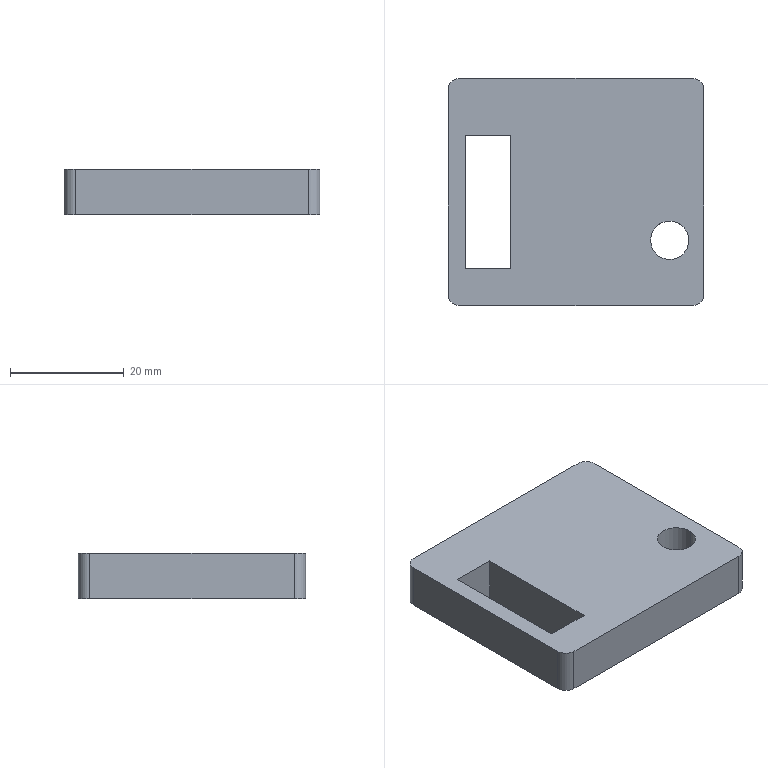Part | SolidWorks | features Fillet 1, FlatPattern 1, SMBaseFlange 1, SheetMetal 1 | 1 solid | 16 faces | box 45 x 40 x 8 mm | volume 12582 mm3 | plane 10 | cylinder 6 | commonest cylinder face diameters 4 x4 6.75 x2
STEP:
#1=CARTESIAN_POINT('',(-158.375,325.,8.));
#2=VERTEX_POINT('',#1);
#3=CARTESIAN_POINT('',(-151.625,325.,8.));
#4=VERTEX_POINT('',#3);
#5=CARTESIAN_POINT('',(-155.,325.,8.));
#6=DIRECTION('',(0.,0.,1.));
#7=DIRECTION('',(1.,0.,0.));
#8=AXIS2_PLACEMENT_3D('',#5,#6,#7);
#9=CIRCLE('',#8,3.375);
#10=EDGE_CURVE('',#2,#4,#9,.T.);
#11=ORIENTED_EDGE('',*,*,#10,.T.);
#12=CARTESIAN_POINT('',(-151.625,325.,0.));
#13=VERTEX_POINT('',#12);
#14=CARTESIAN_POINT('',(-151.625,325.,8.));
#15=DIRECTION('',(0.,0.,-1.));
#16=VECTOR('',#15,1000.);
#17=LINE('',#14,#16);
#18=EDGE_CURVE('',#4,#13,#17,.T.);
#19=ORIENTED_EDGE('',*,*,#18,.T.);
#20=CARTESIAN_POINT('',(-158.375,325.,0.));
#21=VERTEX_POINT('',#20);
#22=CARTESIAN_POINT('',(-155.,325.,0.));
#23=DIRECTION('',(0.,0.,1.));
#24=DIRECTION('',(1.,0.,0.));
#25=AXIS2_PLACEMENT_3D('',#22,#23,#24);
#26=CIRCLE('',#25,3.375);
#27=EDGE_CURVE('',#21,#13,#26,.T.);
#28=ORIENTED_EDGE('',*,*,#27,.F.);
#29=CARTESIAN_POINT('',(-158.375,325.,8.));
#30=DIRECTION('',(0.,0.,-1.));
#31=VECTOR('',#30,1000.);
#32=LINE('',#29,#31);
#33=EDGE_CURVE('',#2,#21,#32,.T.);
#34=ORIENTED_EDGE('',*,*,#33,.F.);
#35=EDGE_LOOP('',(#11,#19,#28,#34));
#36=FACE_OUTER_BOUND('',#35,.T.);
#37=CARTESIAN_POINT('',(-155.,325.,8.));
#38=DIRECTION('',(0.,0.,-1.));
#39=DIRECTION('',(-1.,0.,0.));
#40=AXIS2_PLACEMENT_3D('',#37,#38,#39);
#41=CYLINDRICAL_SURFACE('',#40,3.375);
#42=ADVANCED_FACE('',(#36),#41,.F.);
#43=CARTESIAN_POINT('',(-149.,315.5,8.));
#44=VERTEX_POINT('',#43);
#45=CARTESIAN_POINT('',(-149.,351.5,8.));
#46=VERTEX_POINT('',#45);
#47=CARTESIAN_POINT('',(-149.,313.5,8.));
#48=DIRECTION('',(0.,1.,0.));
#49=VECTOR('',#48,1000.);
#50=LINE('',#47,#49);
#51=EDGE_CURVE('',#44,#46,#50,.T.);
#52=ORIENTED_EDGE('',*,*,#51,.T.);
#53=CARTESIAN_POINT('',(-151.,353.5,8.));
#54=VERTEX_POINT('',#53);
#55=CARTESIAN_POINT('',(-151.,351.5,8.));
#56=DIRECTION('',(0.,0.,1.));
#57=DIRECTION('',(1.,0.,0.));
#58=AXIS2_PLACEMENT_3D('',#55,#56,#57);
#59=CIRCLE('',#58,2.);
#60=EDGE_CURVE('',#46,#54,#59,.T.);
#61=ORIENTED_EDGE('',*,*,#60,.T.);
#62=CARTESIAN_POINT('',(-192.,353.5,8.));
#63=VERTEX_POINT('',#62);
#64=CARTESIAN_POINT('',(-149.,353.5,8.));
#65=DIRECTION('',(-1.,0.,0.));
#66=VECTOR('',#65,1000.);
#67=LINE('',#64,#66);
#68=EDGE_CURVE('',#54,#63,#67,.T.);
#69=ORIENTED_EDGE('',*,*,#68,.T.);
#70=CARTESIAN_POINT('',(-194.,351.5,8.));
#71=VERTEX_POINT('',#70);
#72=CARTESIAN_POINT('',(-192.,351.5,8.));
#73=DIRECTION('',(0.,0.,1.));
#74=DIRECTION('',(1.,0.,0.));
#75=AXIS2_PLACEMENT_3D('',#72,#73,#74);
#76=CIRCLE('',#75,2.);
#77=EDGE_CURVE('',#63,#71,#76,.T.);
#78=ORIENTED_EDGE('',*,*,#77,.T.);
#79=CARTESIAN_POINT('',(-194.,315.5,8.));
#80=VERTEX_POINT('',#79);
#81=CARTESIAN_POINT('',(-194.,353.5,8.));
#82=DIRECTION('',(0.,-1.,0.));
#83=VECTOR('',#82,1000.);
#84=LINE('',#81,#83);
#85=EDGE_CURVE('',#71,#80,#84,.T.);
#86=ORIENTED_EDGE('',*,*,#85,.T.);
#87=CARTESIAN_POINT('',(-192.,313.5,8.));
#88=VERTEX_POINT('',#87);
#89=CARTESIAN_POINT('',(-192.,315.5,8.));
#90=DIRECTION('',(0.,0.,1.));
#91=DIRECTION('',(1.,0.,0.));
#92=AXIS2_PLACEMENT_3D('',#89,#90,#91);
#93=CIRCLE('',#92,2.);
#94=EDGE_CURVE('',#80,#88,#93,.T.);
#95=ORIENTED_EDGE('',*,*,#94,.T.);
#96=CARTESIAN_POINT('',(-151.,313.5,8.));
#97=VERTEX_POINT('',#96);
#98=CARTESIAN_POINT('',(-194.,313.5,8.));
#99=DIRECTION('',(1.,0.,0.));
#100=VECTOR('',#99,1000.);
#101=LINE('',#98,#100);
#102=EDGE_CURVE('',#88,#97,#101,.T.);
#103=ORIENTED_EDGE('',*,*,#102,.T.);
#104=CARTESIAN_POINT('',(-151.,315.5,8.));
#105=DIRECTION('',(0.,0.,1.));
#106=DIRECTION('',(1.,0.,0.));
#107=AXIS2_PLACEMENT_3D('',#104,#105,#106);
#108=CIRCLE('',#107,2.);
#109=EDGE_CURVE('',#97,#44,#108,.T.);
#110=ORIENTED_EDGE('',*,*,#109,.T.);
#111=EDGE_LOOP('',(#52,#61,#69,#78,#86,#95,#103,#110));
#112=FACE_OUTER_BOUND('',#111,.T.);
#113=ORIENTED_EDGE('',*,*,#10,.F.);
#114=CARTESIAN_POINT('',(-155.,325.,8.));
#115=DIRECTION('',(0.,0.,1.));
#116=DIRECTION('',(1.,0.,0.));
#117=AXIS2_PLACEMENT_3D('',#114,#115,#116);
#118=CIRCLE('',#117,3.375);
#119=EDGE_CURVE('',#4,#2,#118,.T.);
#120=ORIENTED_EDGE('',*,*,#119,.F.);
#121=EDGE_LOOP('',(#113,#120));
#122=FACE_BOUND('',#121,.T.);
#123=CARTESIAN_POINT('',(-191.,320.,8.));
#124=VERTEX_POINT('',#123);
#125=CARTESIAN_POINT('',(-183.,320.,8.));
#126=VERTEX_POINT('',#125);
#127=CARTESIAN_POINT('',(-183.,320.,8.));
#128=DIRECTION('',(1.,0.,0.));
#129=VECTOR('',#128,1000.);
#130=LINE('',#127,#129);
#131=EDGE_CURVE('',#124,#126,#130,.T.);
#132=ORIENTED_EDGE('',*,*,#131,.F.);
#133=CARTESIAN_POINT('',(-191.,343.5,8.));
#134=VERTEX_POINT('',#133);
#135=CARTESIAN_POINT('',(-191.,320.,8.));
#136=DIRECTION('',(0.,-1.,0.));
#137=VECTOR('',#136,1000.);
#138=LINE('',#135,#137);
#139=EDGE_CURVE('',#134,#124,#138,.T.);
#140=ORIENTED_EDGE('',*,*,#139,.F.);
#141=CARTESIAN_POINT('',(-183.,343.5,8.));
#142=VERTEX_POINT('',#141);
#143=CARTESIAN_POINT('',(-191.,343.5,8.));
#144=DIRECTION('',(-1.,0.,0.));
#145=VECTOR('',#144,1000.);
#146=LINE('',#143,#145);
#147=EDGE_CURVE('',#142,#134,#146,.T.);
#148=ORIENTED_EDGE('',*,*,#147,.F.);
#149=CARTESIAN_POINT('',(-183.,343.5,8.));
#150=DIRECTION('',(0.,1.,0.));
#151=VECTOR('',#150,1000.);
#152=LINE('',#149,#151);
#153=EDGE_CURVE('',#126,#142,#152,.T.);
#154=ORIENTED_EDGE('',*,*,#153,.F.);
#155=EDGE_LOOP('',(#132,#140,#148,#154));
#156=FACE_BOUND('',#155,.T.);
#157=CARTESIAN_POINT('',(0.,0.,8.));
#158=DIRECTION('',(0.,0.,1.));
#159=DIRECTION('',(1.,0.,0.));
#160=AXIS2_PLACEMENT_3D('',#157,#158,#159);
#161=PLANE('',#160);
#162=ADVANCED_FACE('',(#112,#122,#156),#161,.T.);
#163=ORIENTED_EDGE('',*,*,#27,.T.);
#164=CARTESIAN_POINT('',(-155.,325.,0.));
#165=DIRECTION('',(0.,0.,1.));
#166=DIRECTION('',(1.,0.,0.));
#167=AXIS2_PLACEMENT_3D('',#164,#165,#166);
#168=CIRCLE('',#167,3.375);
#169=EDGE_CURVE('',#13,#21,#168,.T.);
#170=ORIENTED_EDGE('',*,*,#169,.T.);
#171=EDGE_LOOP('',(#163,#170));
#172=FACE_BOUND('',#171,.T.);
#173=CARTESIAN_POINT('',(-151.,353.5,0.));
#174=VERTEX_POINT('',#173);
#175=CARTESIAN_POINT('',(-192.,353.5,0.));
#176=VERTEX_POINT('',#175);
#177=CARTESIAN_POINT('',(-149.,353.5,0.));
#178=DIRECTION('',(-1.,0.,0.));
#179=VECTOR('',#178,1000.);
#180=LINE('',#177,#179);
#181=EDGE_CURVE('',#174,#176,#180,.T.);
#182=ORIENTED_EDGE('',*,*,#181,.F.);
#183=CARTESIAN_POINT('',(-149.,351.5,0.));
#184=VERTEX_POINT('',#183);
#185=CARTESIAN_POINT('',(-151.,351.5,0.));
#186=DIRECTION('',(0.,0.,-1.));
#187=DIRECTION('',(1.,0.,0.));
#188=AXIS2_PLACEMENT_3D('',#185,#186,#187);
#189=CIRCLE('',#188,2.);
#190=EDGE_CURVE('',#174,#184,#189,.T.);
#191=ORIENTED_EDGE('',*,*,#190,.T.);
#192=CARTESIAN_POINT('',(-149.,315.5,0.));
#193=VERTEX_POINT('',#192);
#194=CARTESIAN_POINT('',(-149.,313.5,0.));
#195=DIRECTION('',(0.,1.,0.));
#196=VECTOR('',#195,1000.);
#197=LINE('',#194,#196);
#198=EDGE_CURVE('',#193,#184,#197,.T.);
#199=ORIENTED_EDGE('',*,*,#198,.F.);
#200=CARTESIAN_POINT('',(-151.,313.5,0.));
#201=VERTEX_POINT('',#200);
#202=CARTESIAN_POINT('',(-151.,315.5,0.));
#203=DIRECTION('',(0.,0.,-1.));
#204=DIRECTION('',(1.,0.,0.));
#205=AXIS2_PLACEMENT_3D('',#202,#203,#204);
#206=CIRCLE('',#205,2.);
#207=EDGE_CURVE('',#193,#201,#206,.T.);
#208=ORIENTED_EDGE('',*,*,#207,.T.);
#209=CARTESIAN_POINT('',(-192.,313.5,0.));
#210=VERTEX_POINT('',#209);
#211=CARTESIAN_POINT('',(-194.,313.5,0.));
#212=DIRECTION('',(1.,0.,0.));
#213=VECTOR('',#212,1000.);
#214=LINE('',#211,#213);
#215=EDGE_CURVE('',#210,#201,#214,.T.);
#216=ORIENTED_EDGE('',*,*,#215,.F.);
#217=CARTESIAN_POINT('',(-194.,315.5,0.));
#218=VERTEX_POINT('',#217);
#219=CARTESIAN_POINT('',(-192.,315.5,0.));
#220=DIRECTION('',(0.,0.,-1.));
#221=DIRECTION('',(1.,0.,0.));
#222=AXIS2_PLACEMENT_3D('',#219,#220,#221);
#223=CIRCLE('',#222,2.);
#224=EDGE_CURVE('',#210,#218,#223,.T.);
#225=ORIENTED_EDGE('',*,*,#224,.T.);
#226=CARTESIAN_POINT('',(-194.,351.5,0.));
#227=VERTEX_POINT('',#226);
#228=CARTESIAN_POINT('',(-194.,353.5,0.));
#229=DIRECTION('',(0.,-1.,0.));
#230=VECTOR('',#229,1000.);
#231=LINE('',#228,#230);
#232=EDGE_CURVE('',#227,#218,#231,.T.);
#233=ORIENTED_EDGE('',*,*,#232,.F.);
#234=CARTESIAN_POINT('',(-192.,351.5,0.));
#235=DIRECTION('',(0.,0.,-1.));
#236=DIRECTION('',(1.,0.,0.));
#237=AXIS2_PLACEMENT_3D('',#234,#235,#236);
#238=CIRCLE('',#237,2.);
#239=EDGE_CURVE('',#227,#176,#238,.T.);
#240=ORIENTED_EDGE('',*,*,#239,.T.);
#241=EDGE_LOOP('',(#182,#191,#199,#208,#216,#225,#233,#240));
#242=FACE_OUTER_BOUND('',#241,.T.);
#243=CARTESIAN_POINT('',(-191.,343.5,0.));
#244=VERTEX_POINT('',#243);
#245=CARTESIAN_POINT('',(-191.,320.,0.));
#246=VERTEX_POINT('',#245);
#247=CARTESIAN_POINT('',(-191.,320.,0.));
#248=DIRECTION('',(0.,-1.,0.));
#249=VECTOR('',#248,1000.);
#250=LINE('',#247,#249);
#251=EDGE_CURVE('',#244,#246,#250,.T.);
#252=ORIENTED_EDGE('',*,*,#251,.T.);
#253=CARTESIAN_POINT('',(-183.,320.,0.));
#254=VERTEX_POINT('',#253);
#255=CARTESIAN_POINT('',(-183.,320.,0.));
#256=DIRECTION('',(1.,0.,0.));
#257=VECTOR('',#256,1000.);
#258=LINE('',#255,#257);
#259=EDGE_CURVE('',#246,#254,#258,.T.);
#260=ORIENTED_EDGE('',*,*,#259,.T.);
#261=CARTESIAN_POINT('',(-183.,343.5,0.));
#262=VERTEX_POINT('',#261);
#263=CARTESIAN_POINT('',(-183.,343.5,0.));
#264=DIRECTION('',(0.,1.,0.));
#265=VECTOR('',#264,1000.);
#266=LINE('',#263,#265);
#267=EDGE_CURVE('',#254,#262,#266,.T.);
#268=ORIENTED_EDGE('',*,*,#267,.T.);
#269=CARTESIAN_POINT('',(-191.,343.5,0.));
#270=DIRECTION('',(-1.,0.,0.));
#271=VECTOR('',#270,1000.);
#272=LINE('',#269,#271);
#273=EDGE_CURVE('',#262,#244,#272,.T.);
#274=ORIENTED_EDGE('',*,*,#273,.T.);
#275=EDGE_LOOP('',(#252,#260,#268,#274));
#276=FACE_BOUND('',#275,.T.);
#277=CARTESIAN_POINT('',(0.,0.,0.));
#278=DIRECTION('',(0.,0.,1.));
#279=DIRECTION('',(1.,0.,0.));
#280=AXIS2_PLACEMENT_3D('',#277,#278,#279);
#281=PLANE('',#280);
#282=ADVANCED_FACE('',(#172,#242,#276),#281,.F.);
#283=ORIENTED_EDGE('',*,*,#232,.T.);
#284=CARTESIAN_POINT('',(-194.,315.5,8.));
#285=DIRECTION('',(0.,0.,1.));
#286=VECTOR('',#285,1000.);
#287=LINE('',#284,#286);
#288=EDGE_CURVE('',#218,#80,#287,.T.);
#289=ORIENTED_EDGE('',*,*,#288,.T.);
#290=ORIENTED_EDGE('',*,*,#85,.F.);
#291=CARTESIAN_POINT('',(-194.,351.5,8.));
#292=DIRECTION('',(0.,0.,-1.));
#293=VECTOR('',#292,1000.);
#294=LINE('',#291,#293);
#295=EDGE_CURVE('',#71,#227,#294,.T.);
#296=ORIENTED_EDGE('',*,*,#295,.T.);
#297=EDGE_LOOP('',(#283,#289,#290,#296));
#298=FACE_OUTER_BOUND('',#297,.T.);
#299=CARTESIAN_POINT('',(-194.,353.5,8.));
#300=DIRECTION('',(1.,0.,0.));
#301=DIRECTION('',(0.,1.,0.));
#302=AXIS2_PLACEMENT_3D('',#299,#300,#301);
#303=PLANE('',#302);
#304=ADVANCED_FACE('',(#298),#303,.F.);
#305=ORIENTED_EDGE('',*,*,#215,.T.);
#306=CARTESIAN_POINT('',(-151.,313.5,8.));
#307=DIRECTION('',(0.,0.,1.));
#308=VECTOR('',#307,1000.);
#309=LINE('',#306,#308);
#310=EDGE_CURVE('',#201,#97,#309,.T.);
#311=ORIENTED_EDGE('',*,*,#310,.T.);
#312=ORIENTED_EDGE('',*,*,#102,.F.);
#313=CARTESIAN_POINT('',(-192.,313.5,8.));
#314=DIRECTION('',(0.,0.,-1.));
#315=VECTOR('',#314,1000.);
#316=LINE('',#313,#315);
#317=EDGE_CURVE('',#88,#210,#316,.T.);
#318=ORIENTED_EDGE('',*,*,#317,.T.);
#319=EDGE_LOOP('',(#305,#311,#312,#318));
#320=FACE_OUTER_BOUND('',#319,.T.);
#321=CARTESIAN_POINT('',(-194.,313.5,8.));
#322=DIRECTION('',(0.,1.,0.));
#323=DIRECTION('',(0.,0.,1.));
#324=AXIS2_PLACEMENT_3D('',#321,#322,#323);
#325=PLANE('',#324);
#326=ADVANCED_FACE('',(#320),#325,.F.);
#327=ORIENTED_EDGE('',*,*,#198,.T.);
#328=CARTESIAN_POINT('',(-149.,351.5,8.));
#329=DIRECTION('',(0.,0.,1.));
#330=VECTOR('',#329,1000.);
#331=LINE('',#328,#330);
#332=EDGE_CURVE('',#184,#46,#331,.T.);
#333=ORIENTED_EDGE('',*,*,#332,.T.);
#334=ORIENTED_EDGE('',*,*,#51,.F.);
#335=CARTESIAN_POINT('',(-149.,315.5,8.));
#336=DIRECTION('',(0.,0.,-1.));
#337=VECTOR('',#336,1000.);
#338=LINE('',#335,#337);
#339=EDGE_CURVE('',#44,#193,#338,.T.);
#340=ORIENTED_EDGE('',*,*,#339,.T.);
#341=EDGE_LOOP('',(#327,#333,#334,#340));
#342=FACE_OUTER_BOUND('',#341,.T.);
#343=CARTESIAN_POINT('',(-149.,313.5,8.));
#344=DIRECTION('',(-1.,0.,0.));
#345=DIRECTION('',(0.,0.,1.));
#346=AXIS2_PLACEMENT_3D('',#343,#344,#345);
#347=PLANE('',#346);
#348=ADVANCED_FACE('',(#342),#347,.F.);
#349=ORIENTED_EDGE('',*,*,#68,.F.);
#350=CARTESIAN_POINT('',(-151.,353.5,8.));
#351=DIRECTION('',(0.,0.,-1.));
#352=VECTOR('',#351,1000.);
#353=LINE('',#350,#352);
#354=EDGE_CURVE('',#54,#174,#353,.T.);
#355=ORIENTED_EDGE('',*,*,#354,.T.);
#356=ORIENTED_EDGE('',*,*,#181,.T.);
#357=CARTESIAN_POINT('',(-192.,353.5,8.));
#358=DIRECTION('',(0.,0.,1.));
#359=VECTOR('',#358,1000.);
#360=LINE('',#357,#359);
#361=EDGE_CURVE('',#176,#63,#360,.T.);
#362=ORIENTED_EDGE('',*,*,#361,.T.);
#363=EDGE_LOOP('',(#349,#355,#356,#362));
#364=FACE_OUTER_BOUND('',#363,.T.);
#365=CARTESIAN_POINT('',(-149.,353.5,8.));
#366=DIRECTION('',(0.,-1.,0.));
#367=DIRECTION('',(0.,0.,-1.));
#368=AXIS2_PLACEMENT_3D('',#365,#366,#367);
#369=PLANE('',#368);
#370=ADVANCED_FACE('',(#364),#369,.F.);
#371=ORIENTED_EDGE('',*,*,#18,.F.);
#372=ORIENTED_EDGE('',*,*,#119,.T.);
#373=ORIENTED_EDGE('',*,*,#33,.T.);
#374=ORIENTED_EDGE('',*,*,#169,.F.);
#375=EDGE_LOOP('',(#371,#372,#373,#374));
#376=FACE_OUTER_BOUND('',#375,.T.);
#377=CARTESIAN_POINT('',(-155.,325.,8.));
#378=DIRECTION('',(0.,0.,-1.));
#379=DIRECTION('',(-1.,0.,0.));
#380=AXIS2_PLACEMENT_3D('',#377,#378,#379);
#381=CYLINDRICAL_SURFACE('',#380,3.375);
#382=ADVANCED_FACE('',(#376),#381,.F.);
#383=ORIENTED_EDGE('',*,*,#251,.F.);
#384=CARTESIAN_POINT('',(-191.,343.5,8.));
#385=DIRECTION('',(0.,0.,-1.));
#386=VECTOR('',#385,1000.);
#387=LINE('',#384,#386);
#388=EDGE_CURVE('',#134,#244,#387,.T.);
#389=ORIENTED_EDGE('',*,*,#388,.F.);
#390=ORIENTED_EDGE('',*,*,#139,.T.);
#391=CARTESIAN_POINT('',(-191.,320.,8.));
#392=DIRECTION('',(0.,0.,-1.));
#393=VECTOR('',#392,1000.);
#394=LINE('',#391,#393);
#395=EDGE_CURVE('',#124,#246,#394,.T.);
#396=ORIENTED_EDGE('',*,*,#395,.T.);
#397=EDGE_LOOP('',(#383,#389,#390,#396));
#398=FACE_OUTER_BOUND('',#397,.T.);
#399=CARTESIAN_POINT('',(-191.,320.,8.));
#400=DIRECTION('',(1.,0.,0.));
#401=DIRECTION('',(0.,0.,-1.));
#402=AXIS2_PLACEMENT_3D('',#399,#400,#401);
#403=PLANE('',#402);
#404=ADVANCED_FACE('',(#398),#403,.T.);
#405=ORIENTED_EDGE('',*,*,#259,.F.);
#406=ORIENTED_EDGE('',*,*,#395,.F.);
#407=ORIENTED_EDGE('',*,*,#131,.T.);
#408=CARTESIAN_POINT('',(-183.,320.,8.));
#409=DIRECTION('',(0.,0.,-1.));
#410=VECTOR('',#409,1000.);
#411=LINE('',#408,#410);
#412=EDGE_CURVE('',#126,#254,#411,.T.);
#413=ORIENTED_EDGE('',*,*,#412,.T.);
#414=EDGE_LOOP('',(#405,#406,#407,#413));
#415=FACE_OUTER_BOUND('',#414,.T.);
#416=CARTESIAN_POINT('',(-183.,320.,8.));
#417=DIRECTION('',(0.,1.,0.));
#418=DIRECTION('',(0.,0.,1.));
#419=AXIS2_PLACEMENT_3D('',#416,#417,#418);
#420=PLANE('',#419);
#421=ADVANCED_FACE('',(#415),#420,.T.);
#422=ORIENTED_EDGE('',*,*,#267,.F.);
#423=ORIENTED_EDGE('',*,*,#412,.F.);
#424=ORIENTED_EDGE('',*,*,#153,.T.);
#425=CARTESIAN_POINT('',(-183.,343.5,8.));
#426=DIRECTION('',(0.,0.,-1.));
#427=VECTOR('',#426,1000.);
#428=LINE('',#425,#427);
#429=EDGE_CURVE('',#142,#262,#428,.T.);
#430=ORIENTED_EDGE('',*,*,#429,.T.);
#431=EDGE_LOOP('',(#422,#423,#424,#430));
#432=FACE_OUTER_BOUND('',#431,.T.);
#433=CARTESIAN_POINT('',(-183.,343.5,8.));
#434=DIRECTION('',(-1.,0.,0.));
#435=DIRECTION('',(0.,0.,1.));
#436=AXIS2_PLACEMENT_3D('',#433,#434,#435);
#437=PLANE('',#436);
#438=ADVANCED_FACE('',(#432),#437,.T.);
#439=ORIENTED_EDGE('',*,*,#273,.F.);
#440=ORIENTED_EDGE('',*,*,#429,.F.);
#441=ORIENTED_EDGE('',*,*,#147,.T.);
#442=ORIENTED_EDGE('',*,*,#388,.T.);
#443=EDGE_LOOP('',(#439,#440,#441,#442));
#444=FACE_OUTER_BOUND('',#443,.T.);
#445=CARTESIAN_POINT('',(-191.,343.5,8.));
#446=DIRECTION('',(0.,-1.,0.));
#447=DIRECTION('',(0.,0.,-1.));
#448=AXIS2_PLACEMENT_3D('',#445,#446,#447);
#449=PLANE('',#448);
#450=ADVANCED_FACE('',(#444),#449,.T.);
#451=ORIENTED_EDGE('',*,*,#60,.F.);
#452=ORIENTED_EDGE('',*,*,#332,.F.);
#453=ORIENTED_EDGE('',*,*,#190,.F.);
#454=ORIENTED_EDGE('',*,*,#354,.F.);
#455=EDGE_LOOP('',(#451,#452,#453,#454));
#456=FACE_OUTER_BOUND('',#455,.T.);
#457=CARTESIAN_POINT('',(-151.,351.5,8.));
#458=DIRECTION('',(0.,0.,-1.));
#459=DIRECTION('',(-1.,0.,0.));
#460=AXIS2_PLACEMENT_3D('',#457,#458,#459);
#461=CYLINDRICAL_SURFACE('',#460,2.);
#462=ADVANCED_FACE('',(#456),#461,.T.);
#463=ORIENTED_EDGE('',*,*,#109,.F.);
#464=ORIENTED_EDGE('',*,*,#310,.F.);
#465=ORIENTED_EDGE('',*,*,#207,.F.);
#466=ORIENTED_EDGE('',*,*,#339,.F.);
#467=EDGE_LOOP('',(#463,#464,#465,#466));
#468=FACE_OUTER_BOUND('',#467,.T.);
#469=CARTESIAN_POINT('',(-151.,315.5,8.));
#470=DIRECTION('',(0.,0.,-1.));
#471=DIRECTION('',(-1.,0.,0.));
#472=AXIS2_PLACEMENT_3D('',#469,#470,#471);
#473=CYLINDRICAL_SURFACE('',#472,2.);
#474=ADVANCED_FACE('',(#468),#473,.T.);
#475=ORIENTED_EDGE('',*,*,#94,.F.);
#476=ORIENTED_EDGE('',*,*,#288,.F.);
#477=ORIENTED_EDGE('',*,*,#224,.F.);
#478=ORIENTED_EDGE('',*,*,#317,.F.);
#479=EDGE_LOOP('',(#475,#476,#477,#478));
#480=FACE_OUTER_BOUND('',#479,.T.);
#481=CARTESIAN_POINT('',(-192.,315.5,8.));
#482=DIRECTION('',(0.,0.,-1.));
#483=DIRECTION('',(-1.,0.,0.));
#484=AXIS2_PLACEMENT_3D('',#481,#482,#483);
#485=CYLINDRICAL_SURFACE('',#484,2.);
#486=ADVANCED_FACE('',(#480),#485,.T.);
#487=ORIENTED_EDGE('',*,*,#77,.F.);
#488=ORIENTED_EDGE('',*,*,#361,.F.);
#489=ORIENTED_EDGE('',*,*,#239,.F.);
#490=ORIENTED_EDGE('',*,*,#295,.F.);
#491=EDGE_LOOP('',(#487,#488,#489,#490));
#492=FACE_OUTER_BOUND('',#491,.T.);
#493=CARTESIAN_POINT('',(-192.,351.5,8.));
#494=DIRECTION('',(0.,0.,-1.));
#495=DIRECTION('',(-1.,0.,0.));
#496=AXIS2_PLACEMENT_3D('',#493,#494,#495);
#497=CYLINDRICAL_SURFACE('',#496,2.);
#498=ADVANCED_FACE('',(#492),#497,.T.);
#499=CLOSED_SHELL('',(#42,#162,#282,#304,#326,#348,#370,#382,#404,#421,#438,#450,#462,#474,#486,#498));
#500=MANIFOLD_SOLID_BREP('',#499);
#501=CARTESIAN_POINT('',(0.,0.,0.));
#502=DIRECTION('',(0.,0.,1.));
#503=DIRECTION('',(1.,0.,0.));
#504=AXIS2_PLACEMENT_3D('',#501,#502,#503);
#505=(LENGTH_UNIT()NAMED_UNIT(*)SI_UNIT(.MILLI.,.METRE.));
#506=UNCERTAINTY_MEASURE_WITH_UNIT(LENGTH_MEASURE(0.00001),#505,'','');
#507=(NAMED_UNIT(*)PLANE_ANGLE_UNIT()SI_UNIT($,.RADIAN.));
#508=(NAMED_UNIT(*)SI_UNIT($,.STERADIAN.)SOLID_ANGLE_UNIT());
#509=(GEOMETRIC_REPRESENTATION_CONTEXT(3)GLOBAL_UNCERTAINTY_ASSIGNED_CONTEXT((#506))GLOBAL_UNIT_ASSIGNED_CONTEXT((#505,#507,#508))REPRESENTATION_CONTEXT('',''));
#510=ADVANCED_BREP_SHAPE_REPRESENTATION('',(#500,#504),#509);